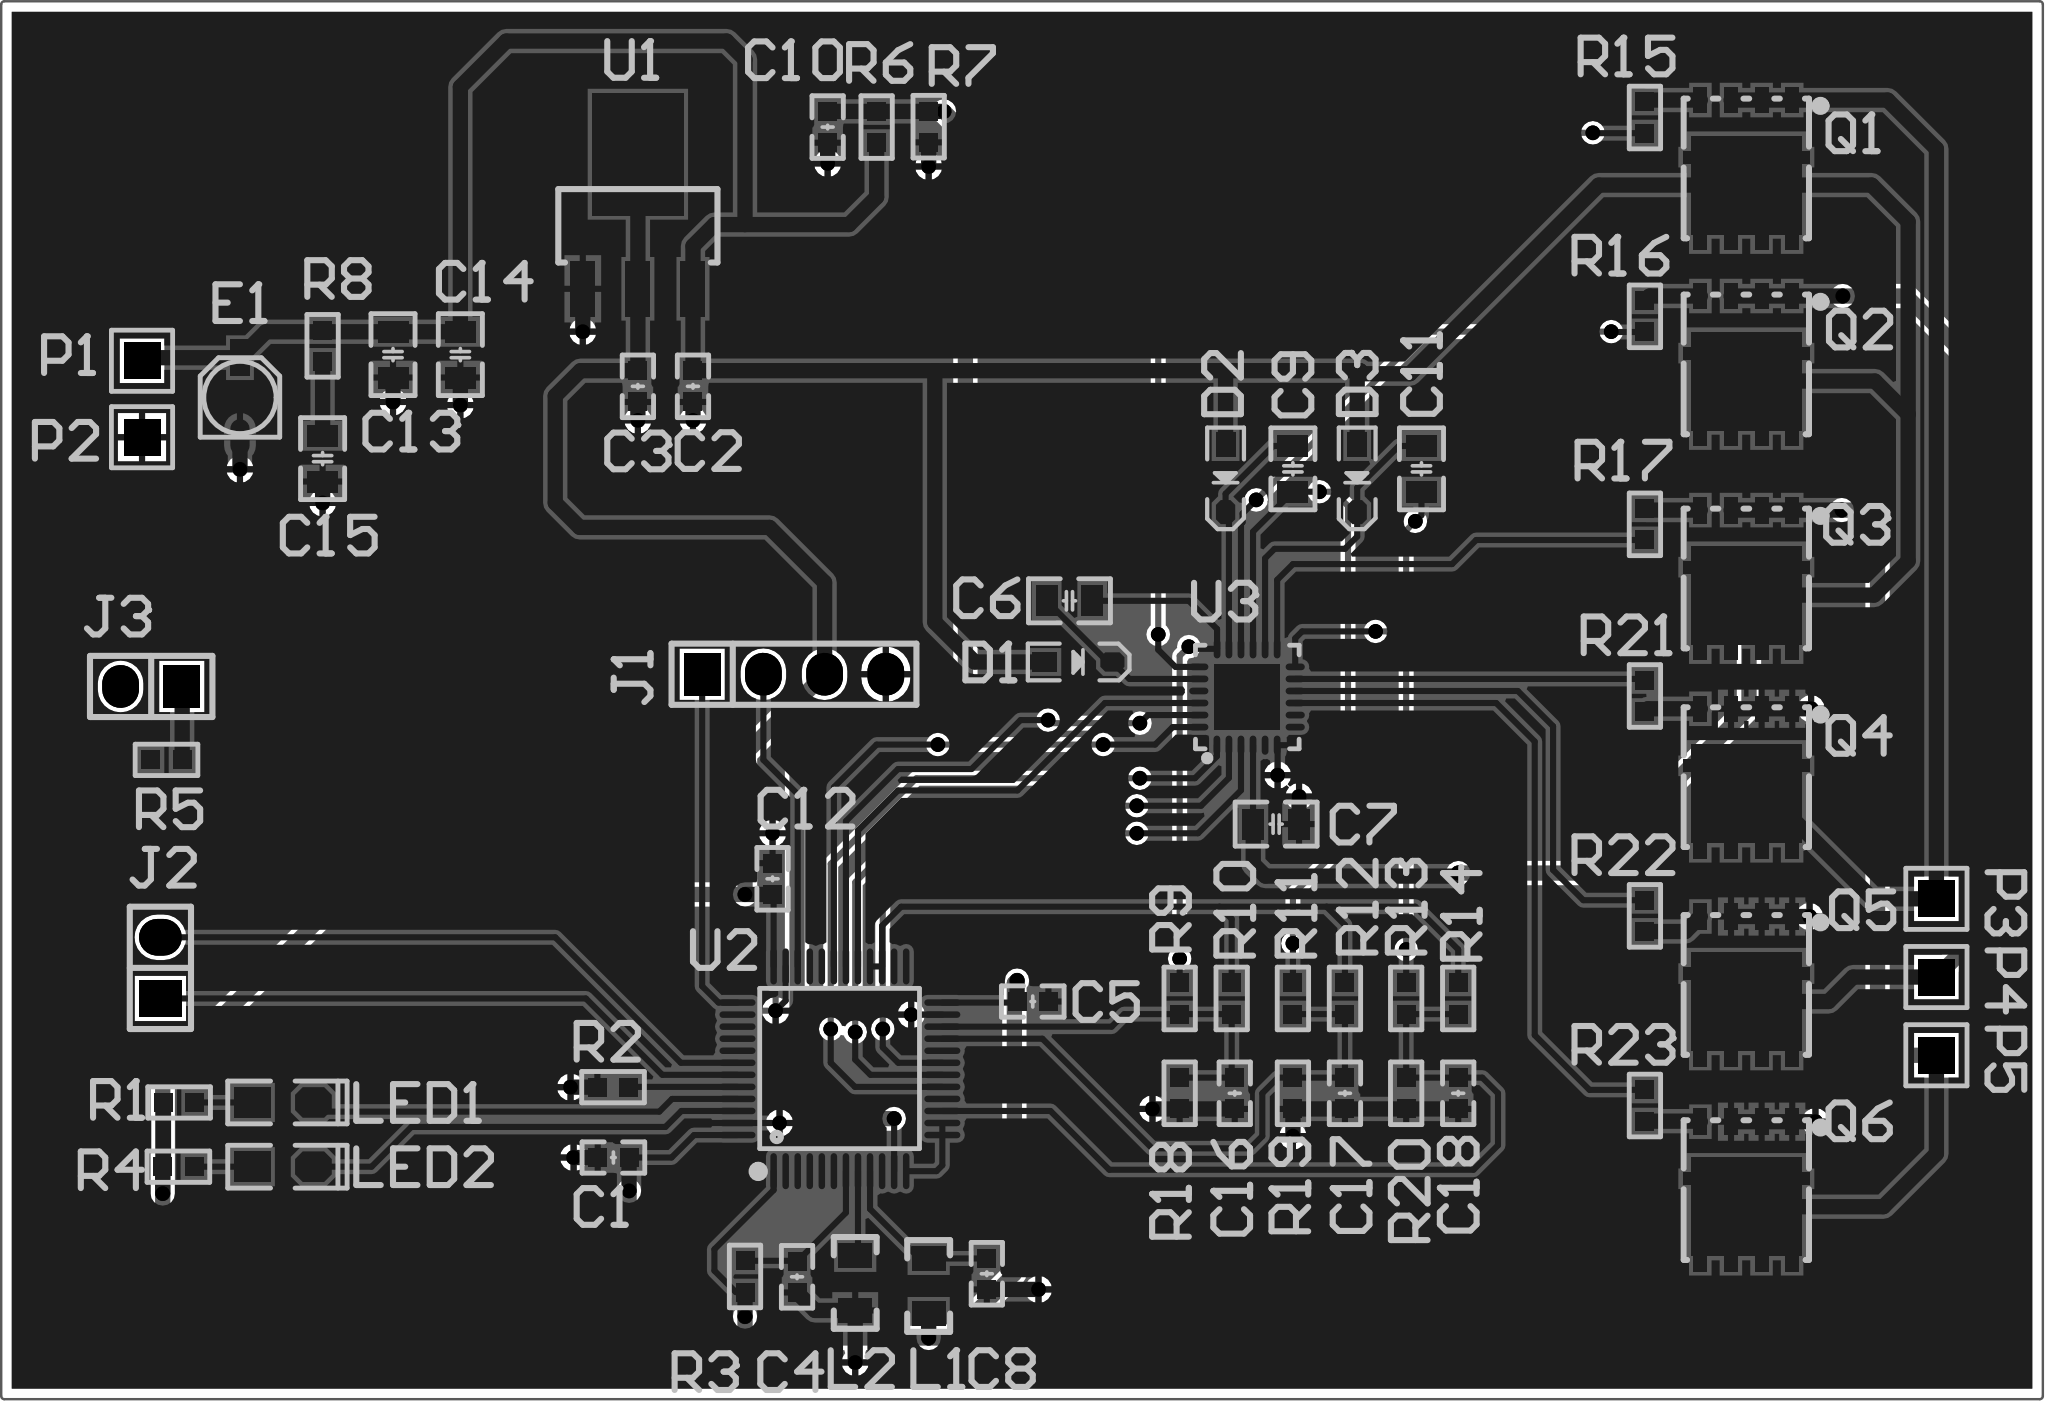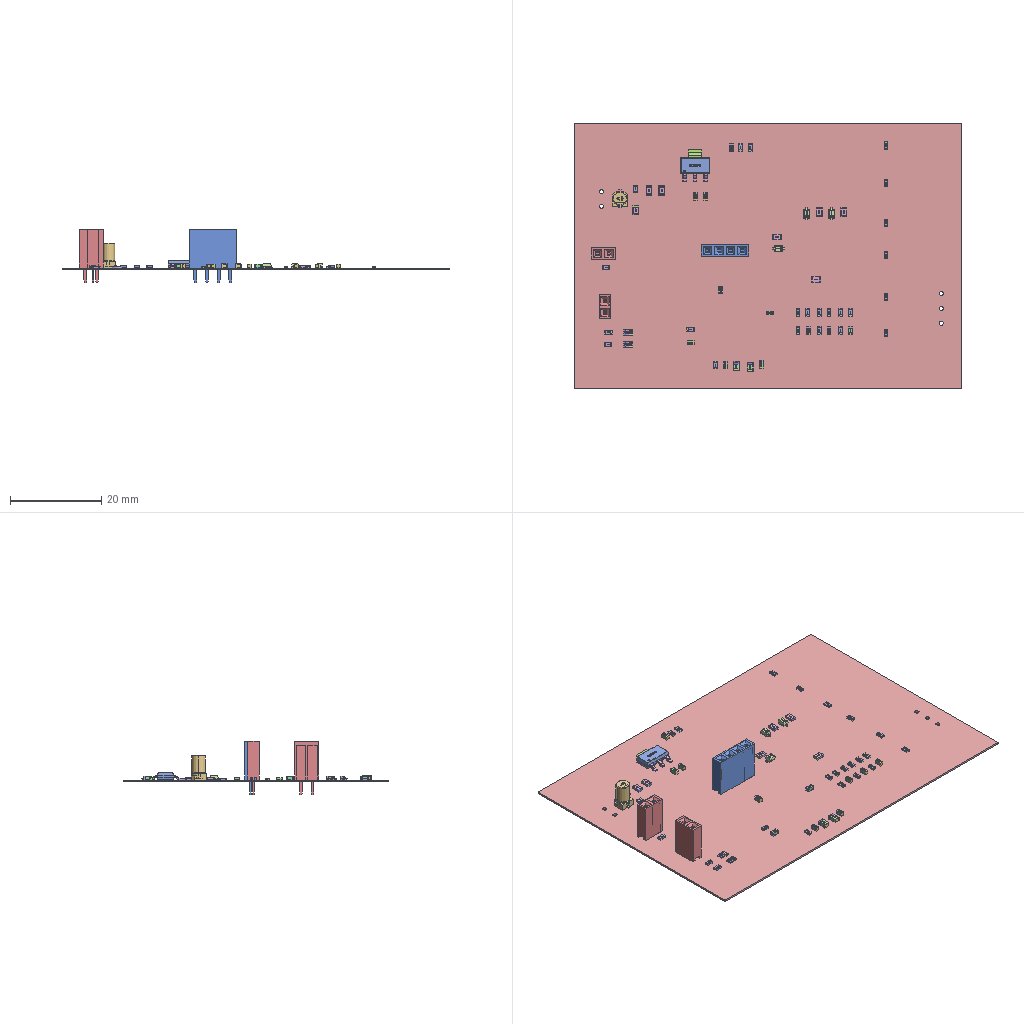Circuit board layout | Altium Designer | box 84.7 x 58 x 11.7 mm
Layer stack:
# Altium Designer layer stack of  (unit mm; dielectric type: 0 none, 1 core, 2 prepreg, 3 surface material)
index,name,kind,layer,copper_thickness_mm,dielectric_type,dielectric_thickness_mm,dielectric_material,dielectric_constant
0,Top Paste,other,,,,,,
1,Top Overlay,other,,,,,,
2,Top Solder,dielectric,,,3,0.0102,Solder Resist,3.5
3,Top Layer,copper,Top Layer,0.0356,,,,
4,Dielectric 1,dielectric,,,0,0.32,FR-4,4.8
5,Bottom Layer,copper,Bottom Layer,0.0356,,,,
6,Bottom Solder,dielectric,,,3,0.0102,Solder Resist,3.5
7,Bottom Overlay,other,,,,,,
8,Bottom Paste,other,,,,,,
# drill layer pairs: low layer,high layer
drill_pair,Top Layer,Bottom Layer
Part placement:
Designator,Comment,Layer,Footprint,Center-X(mm),Center-Y(mm),Rotation
U3,FD6288Q_C7466367,TopLayer,QFN-24_L4.0-W4.0-P0.50-BL-EP2.7,76.962,81.731,360
U2,CH32V203C8T6,TopLayer,LQFP-48_L7.0-W7.0-P0.50-LS9.0-BL,60.071,66.294,0
U1,AMS1117,TopLayer,SOT223,51.689,101.473,0
R23,4.7,TopLayer,R_0603_L,93.472,64.77,90
R22,4.7,TopLayer,R_0603_L,93.472,72.644,90
R21,4.7,TopLayer,R_0603_L,93.472,81.773,90
R20,1K,TopLayer,R_0603_L,83.566,65.278,90
R19,1K,TopLayer,R_0603_L,78.867,65.278,90
R18,1K,TopLayer,R_0603_L,74.168,65.278,90
R17,4.7,TopLayer,R_0603_L,93.472,88.9,270
R16,4.7,TopLayer,R_0603_L,93.472,97.536,270
R15,4.7,TopLayer,R_0603_L,93.472,105.791,270
R14,1K,TopLayer,R_0603_L,85.725,69.215,90
R13,10K,TopLayer,R_0603_L,83.566,69.215,90
R12,1K,TopLayer,R_0603_L,81.026,69.215,90
R11,10K,TopLayer,R_0603_L,78.867,69.215,90
R10,1K,TopLayer,R_0603_L,76.327,69.215,90
R9,10K,TopLayer,R_0603_L,74.168,69.215,90
R8,2,TopLayer,R_0603_L,38.608,96.312,90
R7,10K,TopLayer,R_0603_L,63.754,105.41,90
R6,47K,TopLayer,R_0603_L,61.595,105.395,270
R5,100,TopLayer,R_0603_L,32.131,79.121,180
R4,2.7K,TopLayer,R_0603_L,32.624,62.23,180
R3,10K,TopLayer,R_0603_L,56.134,57.673,270
R2,10K,TopLayer,R_0603_L,50.658,65.532,180
R1,1K,TopLayer,R_0603_L,32.654,64.897,180
Q6,WSD3095DN56,TopLayer,PDFN-8_L5.2-W5.9-P1.27-LS6.2-BL,97.68,61.263,180
Q5,WSD3095DN56,TopLayer,PDFN-8_L5.2-W5.9-P1.27-LS6.2-BL,97.68,69.783,180
Q4,WSD3095DN56,TopLayer,PDFN-8_L5.2-W5.9-P1.27-LS6.2-BL,97.68,78.408,180
Q3,WSD3095DN56,TopLayer,PDFN-8_L5.2-W5.9-P1.27-LS6.2-BL,97.68,86.657,180
Q2,WSD3095DN56,TopLayer,PDFN-8_L5.2-W5.9-P1.27-LS6.2-BL,97.68,95.545,180
Q1,WSD3095DN56,TopLayer,PDFN-8_L5.2-W5.9-P1.27-LS6.2-BL,97.68,103.681,180
P5,HDR1X1,TopLayer,HDR1X1,105.566,66.856,270
P4,HDR1X1,TopLayer,HDR1X1,105.566,70.104,270
P3,HDR1X1,TopLayer,HDR1X1,105.566,73.352,270
P2,HDR1X1,TopLayer,HDR1X1,31.115,92.517,0
P1,HDR1X1,TopLayer,HDR1X1,31.115,95.692,0
LED2,Red,TopLayer,LED_0805G,36.957,62.23,360
LED1,Red,TopLayer,LED_0805G,36.957,64.897,360
L2,10uH,TopLayer,L_0805,60.706,57.404,90
L1,10uH,TopLayer,L_0805,63.754,57.277,90
J3,XH-2AW,TopLayer,Fe-HDR1X2/2.54-S,31.496,82.169,180
J2,Female HDR1X2,TopLayer,Fe-HDR1X2/2.54-S,31.877,70.485,90
J1,Female HDR1X4,TopLayer,Fe-HDR1X4/2.54-S,58.166,82.677,90
E1,470uF,TopLayer,CM_A(3*5.4),35.179,94.169,90
D3,B5819WS,TopLayer,SOD-323,81.534,90.808,270
D2,B5819WS,TopLayer,SOD-323,76.073,90.808,270
D1,B5819WS,TopLayer,SOD-323,69.977,83.185,360
C18,100nF,TopLayer,C_0603_L,85.725,65.278,90
C17,100nF,TopLayer,C_0603_L,81.026,65.278,90
C16,100nF,TopLayer,C_0603_L,76.454,65.278,90
C15,10uF,TopLayer,C_0805_L,38.608,91.628,90
C14,22uF,TopLayer,C_0805_L,44.323,95.946,90
C13,22uF,TopLayer,C_0805_L,41.529,95.946,90
C12,100nF,TopLayer,C_0603_L,57.277,74.183,90
C11,4.7uF,TopLayer,C_0805_L,84.201,91.203,90
C10,100nF,TopLayer,C_0603_L,59.563,105.395,90
C9,4.7uF,TopLayer,C_0805_L,78.867,91.203,90
C8,100nF,TopLayer,C_0603_L,66.167,57.785,90
C7,22uF,TopLayer,C_0805_L,78.171,76.454,180
C6,4.7uF,TopLayer,C_0805_L,69.596,85.725,180
C5,100nF,TopLayer,C_0603_L,68.072,69.088,180
C4,100nF,TopLayer,C_0603_L,58.293,57.658,90
C3,100nF,TopLayer,C_0603_L,51.689,94.63,90
C2,10uF,TopLayer,C_0603_L,53.975,94.63,90
C1,100nF,TopLayer,C_0603_L,50.673,62.611,180
Pad and via stacks:
# Altium Designer via and pad stacks of  (unit mm). Each distinct definition once, with the count of objects using it.
# via: kind,start_layer,end_layer,hole_mm,diameter_mm,mode(0 simple;1 top-mid-bottom;2 full stack),diameter_per_layer,count,example_net
# pad: kind,layer,hole_mm,hole_type(0 round;1 square;2 slot),plating,top_size,top_shape(1 round;2 rect;3 octagon;9 rounded rect),mid_size,bottom_size,mode,footprint,size_per_layer,count,example
pad,Top Layer,0,0,plated,0.762x0.762,2,0.762x0.762,0.762x0.762,0,C 0603_L,,22,C1.1
pad,Top Layer,0,0,plated,1.524x1.27,2,1.524x1.27,1.524x1.27,0,LED 0805G,,2,LED1.1
pad,Top Layer,0,0,plated,1.524x1.27,3,1.524x1.27,1.524x1.27,0,LED 0805G,,2,LED1.2
pad,Top Layer,0,0,plated,0.762x0.762,2,0.762x0.762,0.762x0.762,0,R 0603_L,,46,R1.2
pad,Top Layer,0,0,plated,1.016x2.286,2,1.016x2.286,1.016x2.286,0,SOT223,,3,U1.3
pad,Top Layer,0,0,plated,3.81x5.08,2,3.81x5.08,3.81x5.08,0,SOT223,,1,U1.2
pad,Top Layer,0,0,plated,0.27x1.5,1,0.27x1.5,0.27x1.5,0,LQFP-48_L7.0-W7.0-P0.50-LS9.0-BL,,24,U2.1
pad,Top Layer,0,0,plated,1.5x0.27,1,1.5x0.27,1.5x0.27,0,LQFP-48_L7.0-W7.0-P0.50-LS9.0-BL,,24,U2.13
pad,Top Layer,0,0,plated,0.28x0.8,1,0.28x0.8,0.28x0.8,0,QFN-24_L4.0-W4.0-P0.50-BL-EP2.7,,12,U3.1
pad,Top Layer,0,0,plated,0.8x0.28,1,0.8x0.28,0.8x0.28,0,QFN-24_L4.0-W4.0-P0.50-BL-EP2.7,,12,U3.7
pad,Top Layer,0,0,plated,2.7x2.7,2,2.7x2.7,2.7x2.7,0,QFN-24_L4.0-W4.0-P0.50-BL-EP2.7,,1,U3.25
pad,Top Layer,0,0,plated,1.016x1.397,2,1.016x1.397,1.016x1.397,0,L 0805,,4,L1.2
pad,Top Layer,0,0,plated,1x0.8,3,1x0.8,1x0.8,0,SOD-323,,3,D1.2
pad,Top Layer,0,0,plated,1x0.8,2,1x0.8,1x0.8,0,SOD-323,,3,D1.1
pad,Top Layer,0,0,plated,1.27x0.889,2,1.27x0.889,1.27x0.889,0,C 0805_L,,14,C6.1
pad,Top Layer,0,0,plated,0.58x1.079,2,0.58x1.079,0.58x1.079,0,PDFN-8_L5.2-W5.9-P1.27-LS6.2-BL,,24,Q3.4
pad,Top Layer,0,0,plated,0.58x1.08,2,0.58x1.08,0.58x1.08,0,PDFN-8_L5.2-W5.9-P1.27-LS6.2-BL,,24,Q3.8
pad,Top Layer,0,0,plated,0.95x0.5,2,0.95x0.5,0.95x0.5,0,PDFN-8_L5.2-W5.9-P1.27-LS6.2-BL,,12,Q3.9
pad,Top Layer,0,0,plated,4.6x4.1,2,4.6x4.1,4.6x4.1,0,PDFN-8_L5.2-W5.9-P1.27-LS6.2-BL,,6,Q3.9
pad,Top Layer,0,0,plated,1.5x0.8,2,1.5x0.8,1.5x0.8,0,CM A(3*5.4),,1,E1.1
pad,Top Layer,0,0,plated,1.5x0.8,1,1.5x0.8,1.5x0.8,0,CM A(3*5.4),,1,E1.2
pad,Multi-Layer,0.8128,0,plated,1.524x1.778,1,1.524x1.778,1.524x1.778,0,Fe-HDR1X4/2.54-S,,3,J1.4
pad,Multi-Layer,0.8128,0,plated,1.524x1.778,2,1.524x1.778,1.524x1.778,0,Fe-HDR1X4/2.54-S,,1,J1.1
pad,Multi-Layer,0.8128,0,plated,1.524x1.778,2,1.524x1.778,1.524x1.778,0,Fe-HDR1X2/2.54-S,,2,J2.1
pad,Multi-Layer,0.8128,0,plated,1.524x1.778,1,1.524x1.778,1.524x1.778,0,Fe-HDR1X2/2.54-S,,2,J2.2
pad,Multi-Layer,0.9,2,plated,1.5x1.5,2,1.5x1.5,1.5x1.5,0,HDR1X1,,5,P1.1
via,Top Layer,Bottom Layer,0.3048,0.6096,0,,58,GND
Copper pours:
name,layer,net,type(0 solid;1 hatched;2 none)
D,Bottom Layer,GND,0
D,Top Layer,GND,0
Design rules, without the lines most boards share:
# Altium Designer design rules of  (exported by Altium Designer, unit mm)
# columns: name | kind | enabled | priority | scope1 | scope2 | descriptor | typed fields (field=value)
Clearance | 0 | enabled | 1 | All | All | Clearance Constraint (Gap=7mil) (All),(All) | gap=0.1778
PlaneConnect | 6 | enabled | 1 | All | All | Power Plane Connect Rule(Relief Connect )(Expansion=20mil) (Conductor Width=10mil) (Air Gap=10mil) (Entries=4) (All) | relief_conductor_width=0.254 relief_entries=4 relief_expansion=0.508
PolygonConnect | 20 | enabled | 1 | All | All | Polygon Connect Rule(Relief Connect )(Conductor Width=10mil) (Relief Angle=90 Angle) (Entries=4) (Air Gap Width=10mil) (All),(All) | connect_style(0=relief,1=direct,2=none)=0 relief_conductor_width=0.254 relief_entries=4
Width | 2 | enabled | 1 | All | All | Width Constraint (Min=10mil) (Max=30mil) (Preferred=10mil) (All) |
RoutingVias | 11 | enabled | 1 | All | All | Routing Via (MinHoleWidth=28mil) (MaxHoleWidth=28mil) (PreferredHoleWidth=28mil) (MinWidth=50mil) (MaxWidth=50mil) (PreferedWidth=50mil) (All) | via_min_hole=0.7112 via_max_hole=0.7112 via_preferred_diameter=1.27 via_preferred_hole=0.7112
PasteMaskExpansion | 14 | enabled | 1 | All | All | Paste Mask Expansion (Expansion =0mil) (All) | expansion=0
SolderMaskExpansion | 13 | enabled | 1 | All | All | Solder Mask Expansion (Expansion =4mil) (All) | expansion=0.1016
DiffPairsRouting | 51 | enabled | 1 | All | All | Differential Pairs Uncoupled Length using the Gap Constraints (Min=10mil) (Max=10mil) (Prefered=10mil)  and Width Constraints (Min=15mil) (Max=15mil) (Prefered=15mil) (All) |
HoleToHoleClearance | 52 | enabled | 1 | All | All | Hole To Hole Clearance (Gap=10mil) (All),(All) | gap=0.254
MinimumSolderMaskSliver | 53 | enabled | 1 | All | All | Minimum Solder Mask Sliver (Gap=0mil) (All),(All) |
SilkToSolderMaskClearance | 54 | enabled | 1 | IsPad | All | Silk To Solder Mask (Clearance=0mil) (IsPad),(All) |
SilkToSilkClearance | 55 | enabled | 1 | All | All | Silk to Silk (Clearance=0mil) (All),(All) |
Classes set for this board:
# Altium Designer classes of  (member kind: 0 net, 1 component, 2 from-to, 3 pad, 4 layer, 5 differential pair, 6 design channel, 7 polygon, 8 structure, 9 xSignal)
# columns: class name | member kind | superclass | members
Sheet1 | 1 | no | C1; C2; C3; C4; C5; C6; C7; C8; C9; C10; C11; C12; C13; C14; C15; C16; C17; C18; D1; D2; D3; E1; J1; J2; J3; L1; L2; LED1; LED2; P1; P2; P3; P4; P5; Q1; Q2; Q3; Q4; Q5; Q6; R1; R2; R3; R4; R5; R6; R7; R8; R9; R10; R11; R12; R13; R14; R15; R16; R17; R18; R19; R20; R21; R22; R23; U1; U2; U3;